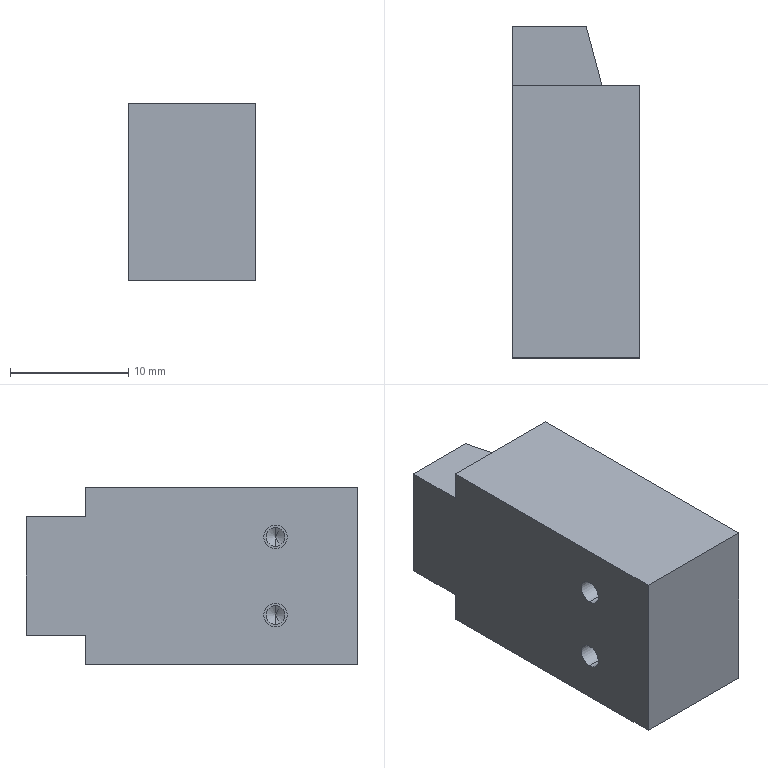Part | STEP file | 11-sy5120-5gz-01_sy51802operend-V2.0-V2.011_SingleA | 1 solid | 27 faces | box 10.8 x 28 x 15 mm | volume 4037 mm3 | plane 13 | cylinder 10 | cone 4 | commonest cylinder face diameters 1.6 x4 2 x4 3.4 x2
STEP:
#1=CARTESIAN_POINT('',(-5.119,6.95,-3.3));
#2=VERTEX_POINT('',#1);
#3=CARTESIAN_POINT('',(-5.6,6.95,-2.5));
#4=VERTEX_POINT('',#3);
#5=CARTESIAN_POINT('',(-5.6,6.95,-2.5));
#6=DIRECTION('',(-0.515,0.,0.8572));
#7=VECTOR('',#6,1000.);
#8=LINE('',#5,#7);
#9=EDGE_CURVE('',#2,#4,#8,.T.);
#10=ORIENTED_EDGE('',*,*,#9,.F.);
#11=CARTESIAN_POINT('',(-5.6,6.95,-4.1));
#12=VERTEX_POINT('',#11);
#13=CARTESIAN_POINT('',(-5.6,6.95,-4.1));
#14=DIRECTION('',(-0.515,0.,-0.8572));
#15=VECTOR('',#14,1000.);
#16=LINE('',#13,#15);
#17=EDGE_CURVE('',#2,#12,#16,.T.);
#18=ORIENTED_EDGE('',*,*,#17,.T.);
#19=CARTESIAN_POINT('',(-5.6,6.95,-3.3));
#20=DIRECTION('',(-1.,0.,0.));
#21=DIRECTION('',(0.,0.,1.));
#22=AXIS2_PLACEMENT_3D('',#19,#20,#21);
#23=CIRCLE('',#22,0.8);
#24=EDGE_CURVE('',#12,#4,#23,.T.);
#25=ORIENTED_EDGE('',*,*,#24,.T.);
#26=EDGE_LOOP('',(#10,#18,#25));
#27=FACE_OUTER_BOUND('',#26,.T.);
#28=CARTESIAN_POINT('',(-5.6,6.95,-3.3));
#29=DIRECTION('',(-1.,0.,0.));
#30=DIRECTION('',(0.,0.,1.));
#31=AXIS2_PLACEMENT_3D('',#28,#29,#30);
#32=CONICAL_SURFACE('',#31,0.8,1.03);
#33=ADVANCED_FACE('',(#27),#32,.F.);
#34=ORIENTED_EDGE('',*,*,#24,.F.);
#35=CARTESIAN_POINT('',(-6.8,6.95,-4.1));
#36=VERTEX_POINT('',#35);
#37=CARTESIAN_POINT('',(-10.8,6.95,-4.1));
#38=DIRECTION('',(-1.,0.,0.));
#39=VECTOR('',#38,1000.);
#40=LINE('',#37,#39);
#41=EDGE_CURVE('',#12,#36,#40,.T.);
#42=ORIENTED_EDGE('',*,*,#41,.T.);
#43=CARTESIAN_POINT('',(-6.8,6.95,-2.5));
#44=VERTEX_POINT('',#43);
#45=CARTESIAN_POINT('',(-6.8,6.95,-3.3));
#46=DIRECTION('',(-1.,0.,0.));
#47=DIRECTION('',(0.,0.,1.));
#48=AXIS2_PLACEMENT_3D('',#45,#46,#47);
#49=CIRCLE('',#48,0.8);
#50=EDGE_CURVE('',#36,#44,#49,.T.);
#51=ORIENTED_EDGE('',*,*,#50,.T.);
#52=CARTESIAN_POINT('',(-10.8,6.95,-2.5));
#53=DIRECTION('',(-1.,0.,0.));
#54=VECTOR('',#53,1000.);
#55=LINE('',#52,#54);
#56=EDGE_CURVE('',#4,#44,#55,.T.);
#57=ORIENTED_EDGE('',*,*,#56,.F.);
#58=EDGE_LOOP('',(#34,#42,#51,#57));
#59=FACE_OUTER_BOUND('',#58,.T.);
#60=CARTESIAN_POINT('',(-10.8,6.95,-3.3));
#61=DIRECTION('',(-1.,0.,0.));
#62=DIRECTION('',(0.,0.,1.));
#63=AXIS2_PLACEMENT_3D('',#60,#61,#62);
#64=CYLINDRICAL_SURFACE('',#63,0.8);
#65=ADVANCED_FACE('',(#59),#64,.F.);
#66=CARTESIAN_POINT('',(-6.8,6.95,-4.3));
#67=VERTEX_POINT('',#66);
#68=CARTESIAN_POINT('',(-6.8,6.95,-2.3));
#69=VERTEX_POINT('',#68);
#70=CARTESIAN_POINT('',(-6.8,6.95,-3.3));
#71=DIRECTION('',(-1.,0.,0.));
#72=DIRECTION('',(0.,0.,1.));
#73=AXIS2_PLACEMENT_3D('',#70,#71,#72);
#74=CIRCLE('',#73,1.);
#75=EDGE_CURVE('',#67,#69,#74,.T.);
#76=ORIENTED_EDGE('',*,*,#75,.F.);
#77=CARTESIAN_POINT('',(-10.8,6.95,-4.3));
#78=VERTEX_POINT('',#77);
#79=CARTESIAN_POINT('',(-10.8,6.95,-4.3));
#80=DIRECTION('',(-1.,0.,0.));
#81=VECTOR('',#80,1000.);
#82=LINE('',#79,#81);
#83=EDGE_CURVE('',#67,#78,#82,.T.);
#84=ORIENTED_EDGE('',*,*,#83,.T.);
#85=CARTESIAN_POINT('',(-10.8,6.95,-2.3));
#86=VERTEX_POINT('',#85);
#87=CARTESIAN_POINT('',(-10.8,6.95,-3.3));
#88=DIRECTION('',(-1.,0.,0.));
#89=DIRECTION('',(0.,0.,1.));
#90=AXIS2_PLACEMENT_3D('',#87,#88,#89);
#91=CIRCLE('',#90,1.);
#92=EDGE_CURVE('',#78,#86,#91,.T.);
#93=ORIENTED_EDGE('',*,*,#92,.T.);
#94=CARTESIAN_POINT('',(-10.8,6.95,-2.3));
#95=DIRECTION('',(-1.,0.,0.));
#96=VECTOR('',#95,1000.);
#97=LINE('',#94,#96);
#98=EDGE_CURVE('',#69,#86,#97,.T.);
#99=ORIENTED_EDGE('',*,*,#98,.F.);
#100=EDGE_LOOP('',(#76,#84,#93,#99));
#101=FACE_OUTER_BOUND('',#100,.T.);
#102=CARTESIAN_POINT('',(-10.8,6.95,-3.3));
#103=DIRECTION('',(-1.,0.,0.));
#104=DIRECTION('',(0.,0.,1.));
#105=AXIS2_PLACEMENT_3D('',#102,#103,#104);
#106=CYLINDRICAL_SURFACE('',#105,1.);
#107=ADVANCED_FACE('',(#101),#106,.F.);
#108=CARTESIAN_POINT('',(-5.119,6.95,3.3));
#109=VERTEX_POINT('',#108);
#110=CARTESIAN_POINT('',(-5.6,6.95,4.1));
#111=VERTEX_POINT('',#110);
#112=CARTESIAN_POINT('',(-5.6,6.95,4.1));
#113=DIRECTION('',(-0.515,0.,0.8572));
#114=VECTOR('',#113,1000.);
#115=LINE('',#112,#114);
#116=EDGE_CURVE('',#109,#111,#115,.T.);
#117=ORIENTED_EDGE('',*,*,#116,.F.);
#118=CARTESIAN_POINT('',(-5.6,6.95,2.5));
#119=VERTEX_POINT('',#118);
#120=CARTESIAN_POINT('',(-5.6,6.95,2.5));
#121=DIRECTION('',(-0.515,0.,-0.8572));
#122=VECTOR('',#121,1000.);
#123=LINE('',#120,#122);
#124=EDGE_CURVE('',#109,#119,#123,.T.);
#125=ORIENTED_EDGE('',*,*,#124,.T.);
#126=CARTESIAN_POINT('',(-5.6,6.95,3.3));
#127=DIRECTION('',(-1.,0.,0.));
#128=DIRECTION('',(0.,0.,1.));
#129=AXIS2_PLACEMENT_3D('',#126,#127,#128);
#130=CIRCLE('',#129,0.8);
#131=EDGE_CURVE('',#119,#111,#130,.T.);
#132=ORIENTED_EDGE('',*,*,#131,.T.);
#133=EDGE_LOOP('',(#117,#125,#132));
#134=FACE_OUTER_BOUND('',#133,.T.);
#135=CARTESIAN_POINT('',(-5.6,6.95,3.3));
#136=DIRECTION('',(-1.,0.,0.));
#137=DIRECTION('',(0.,0.,1.));
#138=AXIS2_PLACEMENT_3D('',#135,#136,#137);
#139=CONICAL_SURFACE('',#138,0.8,1.03);
#140=ADVANCED_FACE('',(#134),#139,.F.);
#141=ORIENTED_EDGE('',*,*,#131,.F.);
#142=CARTESIAN_POINT('',(-6.8,6.95,2.5));
#143=VERTEX_POINT('',#142);
#144=CARTESIAN_POINT('',(-10.8,6.95,2.5));
#145=DIRECTION('',(-1.,0.,0.));
#146=VECTOR('',#145,1000.);
#147=LINE('',#144,#146);
#148=EDGE_CURVE('',#119,#143,#147,.T.);
#149=ORIENTED_EDGE('',*,*,#148,.T.);
#150=CARTESIAN_POINT('',(-6.8,6.95,4.1));
#151=VERTEX_POINT('',#150);
#152=CARTESIAN_POINT('',(-6.8,6.95,3.3));
#153=DIRECTION('',(-1.,0.,0.));
#154=DIRECTION('',(0.,0.,1.));
#155=AXIS2_PLACEMENT_3D('',#152,#153,#154);
#156=CIRCLE('',#155,0.8);
#157=EDGE_CURVE('',#143,#151,#156,.T.);
#158=ORIENTED_EDGE('',*,*,#157,.T.);
#159=CARTESIAN_POINT('',(-10.8,6.95,4.1));
#160=DIRECTION('',(-1.,0.,0.));
#161=VECTOR('',#160,1000.);
#162=LINE('',#159,#161);
#163=EDGE_CURVE('',#111,#151,#162,.T.);
#164=ORIENTED_EDGE('',*,*,#163,.F.);
#165=EDGE_LOOP('',(#141,#149,#158,#164));
#166=FACE_OUTER_BOUND('',#165,.T.);
#167=CARTESIAN_POINT('',(-10.8,6.95,3.3));
#168=DIRECTION('',(-1.,0.,0.));
#169=DIRECTION('',(0.,0.,1.));
#170=AXIS2_PLACEMENT_3D('',#167,#168,#169);
#171=CYLINDRICAL_SURFACE('',#170,0.8);
#172=ADVANCED_FACE('',(#166),#171,.F.);
#173=CARTESIAN_POINT('',(-6.8,6.95,2.3));
#174=VERTEX_POINT('',#173);
#175=CARTESIAN_POINT('',(-6.8,6.95,4.3));
#176=VERTEX_POINT('',#175);
#177=CARTESIAN_POINT('',(-6.8,6.95,3.3));
#178=DIRECTION('',(-1.,0.,0.));
#179=DIRECTION('',(0.,0.,1.));
#180=AXIS2_PLACEMENT_3D('',#177,#178,#179);
#181=CIRCLE('',#180,1.);
#182=EDGE_CURVE('',#174,#176,#181,.T.);
#183=ORIENTED_EDGE('',*,*,#182,.F.);
#184=CARTESIAN_POINT('',(-10.8,6.95,2.3));
#185=VERTEX_POINT('',#184);
#186=CARTESIAN_POINT('',(-10.8,6.95,2.3));
#187=DIRECTION('',(-1.,0.,0.));
#188=VECTOR('',#187,1000.);
#189=LINE('',#186,#188);
#190=EDGE_CURVE('',#174,#185,#189,.T.);
#191=ORIENTED_EDGE('',*,*,#190,.T.);
#192=CARTESIAN_POINT('',(-10.8,6.95,4.3));
#193=VERTEX_POINT('',#192);
#194=CARTESIAN_POINT('',(-10.8,6.95,3.3));
#195=DIRECTION('',(-1.,0.,0.));
#196=DIRECTION('',(0.,0.,1.));
#197=AXIS2_PLACEMENT_3D('',#194,#195,#196);
#198=CIRCLE('',#197,1.);
#199=EDGE_CURVE('',#185,#193,#198,.T.);
#200=ORIENTED_EDGE('',*,*,#199,.T.);
#201=CARTESIAN_POINT('',(-10.8,6.95,4.3));
#202=DIRECTION('',(-1.,0.,0.));
#203=VECTOR('',#202,1000.);
#204=LINE('',#201,#203);
#205=EDGE_CURVE('',#176,#193,#204,.T.);
#206=ORIENTED_EDGE('',*,*,#205,.F.);
#207=EDGE_LOOP('',(#183,#191,#200,#206));
#208=FACE_OUTER_BOUND('',#207,.T.);
#209=CARTESIAN_POINT('',(-10.8,6.95,3.3));
#210=DIRECTION('',(-1.,0.,0.));
#211=DIRECTION('',(0.,0.,1.));
#212=AXIS2_PLACEMENT_3D('',#209,#210,#211);
#213=CYLINDRICAL_SURFACE('',#212,1.);
#214=ADVANCED_FACE('',(#208),#213,.F.);
#215=CARTESIAN_POINT('',(-8.1,27.5,-1.7));
#216=VERTEX_POINT('',#215);
#217=CARTESIAN_POINT('',(-8.1,27.5,1.7));
#218=VERTEX_POINT('',#217);
#219=CARTESIAN_POINT('',(-8.1,27.5,0.));
#220=DIRECTION('',(0.,1.,0.));
#221=DIRECTION('',(0.,0.,1.));
#222=AXIS2_PLACEMENT_3D('',#219,#220,#221);
#223=CIRCLE('',#222,1.7);
#224=EDGE_CURVE('',#216,#218,#223,.T.);
#225=ORIENTED_EDGE('',*,*,#224,.F.);
#226=CARTESIAN_POINT('',(-8.1,28.,-1.7));
#227=VERTEX_POINT('',#226);
#228=CARTESIAN_POINT('',(-8.1,27.5,-1.7));
#229=DIRECTION('',(0.,1.,0.));
#230=VECTOR('',#229,1000.);
#231=LINE('',#228,#230);
#232=EDGE_CURVE('',#216,#227,#231,.T.);
#233=ORIENTED_EDGE('',*,*,#232,.T.);
#234=CARTESIAN_POINT('',(-8.1,28.,1.7));
#235=VERTEX_POINT('',#234);
#236=CARTESIAN_POINT('',(-8.1,28.,0.));
#237=DIRECTION('',(0.,1.,0.));
#238=DIRECTION('',(0.,0.,1.));
#239=AXIS2_PLACEMENT_3D('',#236,#237,#238);
#240=CIRCLE('',#239,1.7);
#241=EDGE_CURVE('',#227,#235,#240,.T.);
#242=ORIENTED_EDGE('',*,*,#241,.T.);
#243=CARTESIAN_POINT('',(-8.1,27.5,1.7));
#244=DIRECTION('',(0.,1.,0.));
#245=VECTOR('',#244,1000.);
#246=LINE('',#243,#245);
#247=EDGE_CURVE('',#218,#235,#246,.T.);
#248=ORIENTED_EDGE('',*,*,#247,.F.);
#249=EDGE_LOOP('',(#225,#233,#242,#248));
#250=FACE_OUTER_BOUND('',#249,.T.);
#251=CARTESIAN_POINT('',(-8.1,27.5,0.));
#252=DIRECTION('',(0.,1.,0.));
#253=DIRECTION('',(0.,0.,1.));
#254=AXIS2_PLACEMENT_3D('',#251,#252,#253);
#255=CYLINDRICAL_SURFACE('',#254,1.7);
#256=ADVANCED_FACE('',(#250),#255,.F.);
#257=CARTESIAN_POINT('',(-10.8,0.,7.5));
#258=VERTEX_POINT('',#257);
#259=CARTESIAN_POINT('',(-10.8,0.,-7.5));
#260=VERTEX_POINT('',#259);
#261=CARTESIAN_POINT('',(-10.8,0.,7.5));
#262=DIRECTION('',(0.,0.,-1.));
#263=VECTOR('',#262,1000.);
#264=LINE('',#261,#263);
#265=EDGE_CURVE('',#258,#260,#264,.T.);
#266=ORIENTED_EDGE('',*,*,#265,.T.);
#267=CARTESIAN_POINT('',(0.,0.,-7.5));
#268=VERTEX_POINT('',#267);
#269=CARTESIAN_POINT('',(-10.8,0.,-7.5));
#270=DIRECTION('',(1.,0.,0.));
#271=VECTOR('',#270,1000.);
#272=LINE('',#269,#271);
#273=EDGE_CURVE('',#260,#268,#272,.T.);
#274=ORIENTED_EDGE('',*,*,#273,.T.);
#275=CARTESIAN_POINT('',(0.,0.,7.5));
#276=VERTEX_POINT('',#275);
#277=CARTESIAN_POINT('',(0.,0.,7.5));
#278=DIRECTION('',(0.,0.,-1.));
#279=VECTOR('',#278,1000.);
#280=LINE('',#277,#279);
#281=EDGE_CURVE('',#276,#268,#280,.T.);
#282=ORIENTED_EDGE('',*,*,#281,.F.);
#283=CARTESIAN_POINT('',(-10.8,0.,7.5));
#284=DIRECTION('',(1.,0.,0.));
#285=VECTOR('',#284,1000.);
#286=LINE('',#283,#285);
#287=EDGE_CURVE('',#258,#276,#286,.T.);
#288=ORIENTED_EDGE('',*,*,#287,.F.);
#289=EDGE_LOOP('',(#266,#274,#282,#288));
#290=FACE_OUTER_BOUND('',#289,.T.);
#291=CARTESIAN_POINT('',(-10.8,0.,7.5));
#292=DIRECTION('',(0.,1.,0.));
#293=DIRECTION('',(0.,0.,1.));
#294=AXIS2_PLACEMENT_3D('',#291,#292,#293);
#295=PLANE('',#294);
#296=ADVANCED_FACE('',(#290),#295,.F.);
#297=ORIENTED_EDGE('',*,*,#281,.T.);
#298=CARTESIAN_POINT('',(0.,23.,-7.5));
#299=VERTEX_POINT('',#298);
#300=CARTESIAN_POINT('',(0.,0.,-7.5));
#301=DIRECTION('',(0.,1.,0.));
#302=VECTOR('',#301,1000.);
#303=LINE('',#300,#302);
#304=EDGE_CURVE('',#268,#299,#303,.T.);
#305=ORIENTED_EDGE('',*,*,#304,.T.);
#306=CARTESIAN_POINT('',(0.,23.,7.5));
#307=VERTEX_POINT('',#306);
#308=CARTESIAN_POINT('',(0.,23.,7.5));
#309=DIRECTION('',(0.,0.,-1.));
#310=VECTOR('',#309,1000.);
#311=LINE('',#308,#310);
#312=EDGE_CURVE('',#307,#299,#311,.T.);
#313=ORIENTED_EDGE('',*,*,#312,.F.);
#314=CARTESIAN_POINT('',(0.,0.,7.5));
#315=DIRECTION('',(0.,1.,0.));
#316=VECTOR('',#315,1000.);
#317=LINE('',#314,#316);
#318=EDGE_CURVE('',#276,#307,#317,.T.);
#319=ORIENTED_EDGE('',*,*,#318,.F.);
#320=EDGE_LOOP('',(#297,#305,#313,#319));
#321=FACE_OUTER_BOUND('',#320,.T.);
#322=CARTESIAN_POINT('',(0.,0.,7.5));
#323=DIRECTION('',(-1.,0.,0.));
#324=DIRECTION('',(0.,-1.,0.));
#325=AXIS2_PLACEMENT_3D('',#322,#323,#324);
#326=PLANE('',#325);
#327=ADVANCED_FACE('',(#321),#326,.F.);
#328=CARTESIAN_POINT('',(-10.8,23.,-5.));
#329=VERTEX_POINT('',#328);
#330=CARTESIAN_POINT('',(-10.8,23.,-7.5));
#331=VERTEX_POINT('',#330);
#332=CARTESIAN_POINT('',(-10.8,23.,7.5));
#333=DIRECTION('',(0.,0.,-1.));
#334=VECTOR('',#333,1000.);
#335=LINE('',#332,#334);
#336=EDGE_CURVE('',#329,#331,#335,.T.);
#337=ORIENTED_EDGE('',*,*,#336,.F.);
#338=CARTESIAN_POINT('',(-3.2,23.,-5.));
#339=VERTEX_POINT('',#338);
#340=CARTESIAN_POINT('',(-3.2,23.,-5.));
#341=DIRECTION('',(1.,0.,0.));
#342=VECTOR('',#341,1000.);
#343=LINE('',#340,#342);
#344=EDGE_CURVE('',#329,#339,#343,.T.);
#345=ORIENTED_EDGE('',*,*,#344,.T.);
#346=CARTESIAN_POINT('',(-3.2,23.,5.));
#347=VERTEX_POINT('',#346);
#348=CARTESIAN_POINT('',(-3.2,23.,5.));
#349=DIRECTION('',(0.,0.,-1.));
#350=VECTOR('',#349,1000.);
#351=LINE('',#348,#350);
#352=EDGE_CURVE('',#347,#339,#351,.T.);
#353=ORIENTED_EDGE('',*,*,#352,.F.);
#354=CARTESIAN_POINT('',(-10.8,23.,5.));
#355=VERTEX_POINT('',#354);
#356=CARTESIAN_POINT('',(-3.2,23.,5.));
#357=DIRECTION('',(1.,0.,0.));
#358=VECTOR('',#357,1000.);
#359=LINE('',#356,#358);
#360=EDGE_CURVE('',#355,#347,#359,.T.);
#361=ORIENTED_EDGE('',*,*,#360,.F.);
#362=CARTESIAN_POINT('',(-10.8,23.,7.5));
#363=VERTEX_POINT('',#362);
#364=CARTESIAN_POINT('',(-10.8,23.,7.5));
#365=DIRECTION('',(0.,0.,-1.));
#366=VECTOR('',#365,1000.);
#367=LINE('',#364,#366);
#368=EDGE_CURVE('',#363,#355,#367,.T.);
#369=ORIENTED_EDGE('',*,*,#368,.F.);
#370=CARTESIAN_POINT('',(0.,23.,7.5));
#371=DIRECTION('',(-1.,0.,0.));
#372=VECTOR('',#371,1000.);
#373=LINE('',#370,#372);
#374=EDGE_CURVE('',#307,#363,#373,.T.);
#375=ORIENTED_EDGE('',*,*,#374,.F.);
#376=ORIENTED_EDGE('',*,*,#312,.T.);
#377=CARTESIAN_POINT('',(0.,23.,-7.5));
#378=DIRECTION('',(-1.,0.,0.));
#379=VECTOR('',#378,1000.);
#380=LINE('',#377,#379);
#381=EDGE_CURVE('',#299,#331,#380,.T.);
#382=ORIENTED_EDGE('',*,*,#381,.T.);
#383=EDGE_LOOP('',(#337,#345,#353,#361,#369,#375,#376,#382));
#384=FACE_OUTER_BOUND('',#383,.T.);
#385=CARTESIAN_POINT('',(0.,23.,7.5));
#386=DIRECTION('',(0.,-1.,0.));
#387=DIRECTION('',(1.,0.,0.));
#388=AXIS2_PLACEMENT_3D('',#385,#386,#387);
#389=PLANE('',#388);
#390=ADVANCED_FACE('',(#384),#389,.F.);
#391=CARTESIAN_POINT('',(-10.8,6.95,-3.3));
#392=DIRECTION('',(-1.,0.,0.));
#393=DIRECTION('',(0.,0.,1.));
#394=AXIS2_PLACEMENT_3D('',#391,#392,#393);
#395=CIRCLE('',#394,1.);
#396=EDGE_CURVE('',#86,#78,#395,.T.);
#397=ORIENTED_EDGE('',*,*,#396,.F.);
#398=ORIENTED_EDGE('',*,*,#92,.F.);
#399=EDGE_LOOP('',(#397,#398));
#400=FACE_BOUND('',#399,.T.);
#401=CARTESIAN_POINT('',(-10.8,6.95,3.3));
#402=DIRECTION('',(-1.,0.,0.));
#403=DIRECTION('',(0.,0.,1.));
#404=AXIS2_PLACEMENT_3D('',#401,#402,#403);
#405=CIRCLE('',#404,1.);
#406=EDGE_CURVE('',#193,#185,#405,.T.);
#407=ORIENTED_EDGE('',*,*,#406,.F.);
#408=ORIENTED_EDGE('',*,*,#199,.F.);
#409=EDGE_LOOP('',(#407,#408));
#410=FACE_BOUND('',#409,.T.);
#411=ORIENTED_EDGE('',*,*,#368,.T.);
#412=CARTESIAN_POINT('',(-10.8,28.,5.));
#413=VERTEX_POINT('',#412);
#414=CARTESIAN_POINT('',(-10.8,23.,5.));
#415=DIRECTION('',(0.,-1.,0.));
#416=VECTOR('',#415,1000.);
#417=LINE('',#414,#416);
#418=EDGE_CURVE('',#413,#355,#417,.T.);
#419=ORIENTED_EDGE('',*,*,#418,.F.);
#420=CARTESIAN_POINT('',(-10.8,28.,-5.));
#421=VERTEX_POINT('',#420);
#422=CARTESIAN_POINT('',(-10.8,28.,5.));
#423=DIRECTION('',(0.,0.,-1.));
#424=VECTOR('',#423,1000.);
#425=LINE('',#422,#424);
#426=EDGE_CURVE('',#413,#421,#425,.T.);
#427=ORIENTED_EDGE('',*,*,#426,.T.);
#428=CARTESIAN_POINT('',(-10.8,23.,-5.));
#429=DIRECTION('',(0.,-1.,0.));
#430=VECTOR('',#429,1000.);
#431=LINE('',#428,#430);
#432=EDGE_CURVE('',#421,#329,#431,.T.);
#433=ORIENTED_EDGE('',*,*,#432,.T.);
#434=ORIENTED_EDGE('',*,*,#336,.T.);
#435=CARTESIAN_POINT('',(-10.8,23.,-7.5));
#436=DIRECTION('',(0.,-1.,0.));
#437=VECTOR('',#436,1000.);
#438=LINE('',#435,#437);
#439=EDGE_CURVE('',#331,#260,#438,.T.);
#440=ORIENTED_EDGE('',*,*,#439,.T.);
#441=ORIENTED_EDGE('',*,*,#265,.F.);
#442=CARTESIAN_POINT('',(-10.8,23.,7.5));
#443=DIRECTION('',(0.,-1.,0.));
#444=VECTOR('',#443,1000.);
#445=LINE('',#442,#444);
#446=EDGE_CURVE('',#363,#258,#445,.T.);
#447=ORIENTED_EDGE('',*,*,#446,.F.);
#448=EDGE_LOOP('',(#411,#419,#427,#433,#434,#440,#441,#447));
#449=FACE_OUTER_BOUND('',#448,.T.);
#450=CARTESIAN_POINT('',(-10.8,23.,7.5));
#451=DIRECTION('',(1.,0.,0.));
#452=DIRECTION('',(0.,1.,0.));
#453=AXIS2_PLACEMENT_3D('',#450,#451,#452);
#454=PLANE('',#453);
#455=ADVANCED_FACE('',(#400,#410,#449),#454,.F.);
#456=ORIENTED_EDGE('',*,*,#287,.T.);
#457=ORIENTED_EDGE('',*,*,#318,.T.);
#458=ORIENTED_EDGE('',*,*,#374,.T.);
#459=ORIENTED_EDGE('',*,*,#446,.T.);
#460=EDGE_LOOP('',(#456,#457,#458,#459));
#461=FACE_OUTER_BOUND('',#460,.T.);
#462=CARTESIAN_POINT('',(-10.8,0.,7.5));
#463=DIRECTION('',(0.,0.,-1.));
#464=DIRECTION('',(-1.,0.,0.));
#465=AXIS2_PLACEMENT_3D('',#462,#463,#464);
#466=PLANE('',#465);
#467=ADVANCED_FACE('',(#461),#466,.F.);
#468=ORIENTED_EDGE('',*,*,#273,.F.);
#469=ORIENTED_EDGE('',*,*,#439,.F.);
#470=ORIENTED_EDGE('',*,*,#381,.F.);
#471=ORIENTED_EDGE('',*,*,#304,.F.);
#472=EDGE_LOOP('',(#468,#469,#470,#471));
#473=FACE_OUTER_BOUND('',#472,.T.);
#474=CARTESIAN_POINT('',(-10.8,0.,-7.5));
#475=DIRECTION('',(0.,0.,-1.));
#476=DIRECTION('',(-1.,0.,0.));
#477=AXIS2_PLACEMENT_3D('',#474,#475,#476);
#478=PLANE('',#477);
#479=ADVANCED_FACE('',(#473),#478,.T.);
#480=CARTESIAN_POINT('',(-4.54,28.,-5.));
#481=VERTEX_POINT('',#480);
#482=CARTESIAN_POINT('',(-4.54,28.,-5.));
#483=DIRECTION('',(-0.2588,0.9659,0.));
#484=VECTOR('',#483,1000.);
#485=LINE('',#482,#484);
#486=EDGE_CURVE('',#339,#481,#485,.T.);
#487=ORIENTED_EDGE('',*,*,#486,.T.);
#488=CARTESIAN_POINT('',(-4.54,28.,5.));
#489=VERTEX_POINT('',#488);
#490=CARTESIAN_POINT('',(-4.54,28.,5.));
#491=DIRECTION('',(0.,0.,-1.));
#492=VECTOR('',#491,1000.);
#493=LINE('',#490,#492);
#494=EDGE_CURVE('',#489,#481,#493,.T.);
#495=ORIENTED_EDGE('',*,*,#494,.F.);
#496=CARTESIAN_POINT('',(-4.54,28.,5.));
#497=DIRECTION('',(-0.2588,0.9659,0.));
#498=VECTOR('',#497,1000.);
#499=LINE('',#496,#498);
#500=EDGE_CURVE('',#347,#489,#499,.T.);
#501=ORIENTED_EDGE('',*,*,#500,.F.);
#502=ORIENTED_EDGE('',*,*,#352,.T.);
#503=EDGE_LOOP('',(#487,#495,#501,#502));
#504=FACE_OUTER_BOUND('',#503,.T.);
#505=CARTESIAN_POINT('',(-4.54,28.,5.));
#506=DIRECTION('',(-0.9659,-0.2588,0.));
#507=DIRECTION('',(0.2588,-0.9659,0.));
#508=AXIS2_PLACEMENT_3D('',#505,#506,#507);
#509=PLANE('',#508);
#510=ADVANCED_FACE('',(#504),#509,.F.);
#511=CARTESIAN_POINT('',(-8.1,28.,0.));
#512=DIRECTION('',(0.,1.,0.));
#513=DIRECTION('',(0.,0.,1.));
#514=AXIS2_PLACEMENT_3D('',#511,#512,#513);
#515=CIRCLE('',#514,1.7);
#516=EDGE_CURVE('',#235,#227,#515,.T.);
#517=ORIENTED_EDGE('',*,*,#516,.F.);
#518=ORIENTED_EDGE('',*,*,#241,.F.);
#519=EDGE_LOOP('',(#517,#518));
#520=FACE_BOUND('',#519,.T.);
#521=CARTESIAN_POINT('',(-10.8,28.,-5.));
#522=DIRECTION('',(-1.,0.,0.));
#523=VECTOR('',#522,1000.);
#524=LINE('',#521,#523);
#525=EDGE_CURVE('',#481,#421,#524,.T.);
#526=ORIENTED_EDGE('',*,*,#525,.T.);
#527=ORIENTED_EDGE('',*,*,#426,.F.);
#528=CARTESIAN_POINT('',(-10.8,28.,5.));
#529=DIRECTION('',(-1.,0.,0.));
#530=VECTOR('',#529,1000.);
#531=LINE('',#528,#530);
#532=EDGE_CURVE('',#489,#413,#531,.T.);
#533=ORIENTED_EDGE('',*,*,#532,.F.);
#534=ORIENTED_EDGE('',*,*,#494,.T.);
#535=EDGE_LOOP('',(#526,#527,#533,#534));
#536=FACE_OUTER_BOUND('',#535,.T.);
#537=CARTESIAN_POINT('',(-10.8,28.,5.));
#538=DIRECTION('',(0.,-1.,0.));
#539=DIRECTION('',(1.,0.,0.));
#540=AXIS2_PLACEMENT_3D('',#537,#538,#539);
#541=PLANE('',#540);
#542=ADVANCED_FACE('',(#520,#536),#541,.F.);
#543=ORIENTED_EDGE('',*,*,#418,.T.);
#544=ORIENTED_EDGE('',*,*,#360,.T.);
#545=ORIENTED_EDGE('',*,*,#500,.T.);
#546=ORIENTED_EDGE('',*,*,#532,.T.);
#547=EDGE_LOOP('',(#543,#544,#545,#546));
#548=FACE_OUTER_BOUND('',#547,.T.);
#549=CARTESIAN_POINT('',(-10.8,28.,5.));
#550=DIRECTION('',(0.,0.,-1.));
#551=DIRECTION('',(-1.,0.,0.));
#552=AXIS2_PLACEMENT_3D('',#549,#550,#551);
#553=PLANE('',#552);
#554=ADVANCED_FACE('',(#548),#553,.F.);
#555=ORIENTED_EDGE('',*,*,#432,.F.);
#556=ORIENTED_EDGE('',*,*,#525,.F.);
#557=ORIENTED_EDGE('',*,*,#486,.F.);
#558=ORIENTED_EDGE('',*,*,#344,.F.);
#559=EDGE_LOOP('',(#555,#556,#557,#558));
#560=FACE_OUTER_BOUND('',#559,.T.);
#561=CARTESIAN_POINT('',(-10.8,28.,-5.));
#562=DIRECTION('',(0.,0.,-1.));
#563=DIRECTION('',(-1.,0.,0.));
#564=AXIS2_PLACEMENT_3D('',#561,#562,#563);
#565=PLANE('',#564);
#566=ADVANCED_FACE('',(#560),#565,.T.);
#567=ORIENTED_EDGE('',*,*,#232,.F.);
#568=CARTESIAN_POINT('',(-8.1,27.5,0.));
#569=DIRECTION('',(0.,1.,0.));
#570=DIRECTION('',(0.,0.,1.));
#571=AXIS2_PLACEMENT_3D('',#568,#569,#570);
#572=CIRCLE('',#571,1.7);
#573=EDGE_CURVE('',#218,#216,#572,.T.);
#574=ORIENTED_EDGE('',*,*,#573,.F.);
#575=ORIENTED_EDGE('',*,*,#247,.T.);
#576=ORIENTED_EDGE('',*,*,#516,.T.);
#577=EDGE_LOOP('',(#567,#574,#575,#576));
#578=FACE_OUTER_BOUND('',#577,.T.);
#579=CARTESIAN_POINT('',(-8.1,27.5,0.));
#580=DIRECTION('',(0.,1.,0.));
#581=DIRECTION('',(0.,0.,1.));
#582=AXIS2_PLACEMENT_3D('',#579,#580,#581);
#583=CYLINDRICAL_SURFACE('',#582,1.7);
#584=ADVANCED_FACE('',(#578),#583,.F.);
#585=ORIENTED_EDGE('',*,*,#573,.T.);
#586=ORIENTED_EDGE('',*,*,#224,.T.);
#587=EDGE_LOOP('',(#585,#586));
#588=FACE_OUTER_BOUND('',#587,.T.);
#589=CARTESIAN_POINT('',(-8.1,27.5,0.));
#590=DIRECTION('',(0.,1.,0.));
#591=DIRECTION('',(0.,0.,1.));
#592=AXIS2_PLACEMENT_3D('',#589,#590,#591);
#593=PLANE('',#592);
#594=ADVANCED_FACE('',(#588),#593,.T.);
#595=ORIENTED_EDGE('',*,*,#190,.F.);
#596=CARTESIAN_POINT('',(-6.8,6.95,3.3));
#597=DIRECTION('',(-1.,0.,0.));
#598=DIRECTION('',(0.,0.,1.));
#599=AXIS2_PLACEMENT_3D('',#596,#597,#598);
#600=CIRCLE('',#599,1.);
#601=EDGE_CURVE('',#176,#174,#600,.T.);
#602=ORIENTED_EDGE('',*,*,#601,.F.);
#603=ORIENTED_EDGE('',*,*,#205,.T.);
#604=ORIENTED_EDGE('',*,*,#406,.T.);
#605=EDGE_LOOP('',(#595,#602,#603,#604));
#606=FACE_OUTER_BOUND('',#605,.T.);
#607=CARTESIAN_POINT('',(-10.8,6.95,3.3));
#608=DIRECTION('',(-1.,0.,0.));
#609=DIRECTION('',(0.,0.,1.));
#610=AXIS2_PLACEMENT_3D('',#607,#608,#609);
#611=CYLINDRICAL_SURFACE('',#610,1.);
#612=ADVANCED_FACE('',(#606),#611,.F.);
#613=CARTESIAN_POINT('',(-6.8,6.95,3.3));
#614=DIRECTION('',(-1.,0.,0.));
#615=DIRECTION('',(0.,0.,1.));
#616=AXIS2_PLACEMENT_3D('',#613,#614,#615);
#617=CIRCLE('',#616,0.8);
#618=EDGE_CURVE('',#151,#143,#617,.T.);
#619=ORIENTED_EDGE('',*,*,#618,.F.);
#620=ORIENTED_EDGE('',*,*,#157,.F.);
#621=EDGE_LOOP('',(#619,#620));
#622=FACE_BOUND('',#621,.T.);
#623=ORIENTED_EDGE('',*,*,#601,.T.);
#624=ORIENTED_EDGE('',*,*,#182,.T.);
#625=EDGE_LOOP('',(#623,#624));
#626=FACE_OUTER_BOUND('',#625,.T.);
#627=CARTESIAN_POINT('',(-6.8,7.75,3.3));
#628=DIRECTION('',(1.,0.,0.));
#629=DIRECTION('',(0.,0.,-1.));
#630=AXIS2_PLACEMENT_3D('',#627,#628,#629);
#631=PLANE('',#630);
#632=ADVANCED_FACE('',(#622,#626),#631,.F.);
#633=ORIENTED_EDGE('',*,*,#148,.F.);
#634=CARTESIAN_POINT('',(-5.6,6.95,3.3));
#635=DIRECTION('',(-1.,0.,0.));
#636=DIRECTION('',(0.,0.,1.));
#637=AXIS2_PLACEMENT_3D('',#634,#635,#636);
#638=CIRCLE('',#637,0.8);
#639=EDGE_CURVE('',#111,#119,#638,.T.);
#640=ORIENTED_EDGE('',*,*,#639,.F.);
#641=ORIENTED_EDGE('',*,*,#163,.T.);
#642=ORIENTED_EDGE('',*,*,#618,.T.);
#643=EDGE_LOOP('',(#633,#640,#641,#642));
#644=FACE_OUTER_BOUND('',#643,.T.);
#645=CARTESIAN_POINT('',(-10.8,6.95,3.3));
#646=DIRECTION('',(-1.,0.,0.));
#647=DIRECTION('',(0.,0.,1.));
#648=AXIS2_PLACEMENT_3D('',#645,#646,#647);
#649=CYLINDRICAL_SURFACE('',#648,0.8);
#650=ADVANCED_FACE('',(#644),#649,.F.);
#651=ORIENTED_EDGE('',*,*,#124,.F.);
#652=ORIENTED_EDGE('',*,*,#116,.T.);
#653=ORIENTED_EDGE('',*,*,#639,.T.);
#654=EDGE_LOOP('',(#651,#652,#653));
#655=FACE_OUTER_BOUND('',#654,.T.);
#656=CARTESIAN_POINT('',(-5.6,6.95,3.3));
#657=DIRECTION('',(-1.,0.,0.));
#658=DIRECTION('',(0.,0.,1.));
#659=AXIS2_PLACEMENT_3D('',#656,#657,#658);
#660=CONICAL_SURFACE('',#659,0.8,1.03);
#661=ADVANCED_FACE('',(#655),#660,.F.);
#662=ORIENTED_EDGE('',*,*,#83,.F.);
#663=CARTESIAN_POINT('',(-6.8,6.95,-3.3));
#664=DIRECTION('',(-1.,0.,0.));
#665=DIRECTION('',(0.,0.,1.));
#666=AXIS2_PLACEMENT_3D('',#663,#664,#665);
#667=CIRCLE('',#666,1.);
#668=EDGE_CURVE('',#69,#67,#667,.T.);
#669=ORIENTED_EDGE('',*,*,#668,.F.);
#670=ORIENTED_EDGE('',*,*,#98,.T.);
#671=ORIENTED_EDGE('',*,*,#396,.T.);
#672=EDGE_LOOP('',(#662,#669,#670,#671));
#673=FACE_OUTER_BOUND('',#672,.T.);
#674=CARTESIAN_POINT('',(-10.8,6.95,-3.3));
#675=DIRECTION('',(-1.,0.,0.));
#676=DIRECTION('',(0.,0.,1.));
#677=AXIS2_PLACEMENT_3D('',#674,#675,#676);
#678=CYLINDRICAL_SURFACE('',#677,1.);
#679=ADVANCED_FACE('',(#673),#678,.F.);
#680=CARTESIAN_POINT('',(-6.8,6.95,-3.3));
#681=DIRECTION('',(-1.,0.,0.));
#682=DIRECTION('',(0.,0.,1.));
#683=AXIS2_PLACEMENT_3D('',#680,#681,#682);
#684=CIRCLE('',#683,0.8);
#685=EDGE_CURVE('',#44,#36,#684,.T.);
#686=ORIENTED_EDGE('',*,*,#685,.F.);
#687=ORIENTED_EDGE('',*,*,#50,.F.);
#688=EDGE_LOOP('',(#686,#687));
#689=FACE_BOUND('',#688,.T.);
#690=ORIENTED_EDGE('',*,*,#668,.T.);
#691=ORIENTED_EDGE('',*,*,#75,.T.);
#692=EDGE_LOOP('',(#690,#691));
#693=FACE_OUTER_BOUND('',#692,.T.);
#694=CARTESIAN_POINT('',(-6.8,7.75,-3.3));
#695=DIRECTION('',(1.,0.,0.));
#696=DIRECTION('',(0.,0.,-1.));
#697=AXIS2_PLACEMENT_3D('',#694,#695,#696);
#698=PLANE('',#697);
#699=ADVANCED_FACE('',(#689,#693),#698,.F.);
#700=ORIENTED_EDGE('',*,*,#41,.F.);
#701=CARTESIAN_POINT('',(-5.6,6.95,-3.3));
#702=DIRECTION('',(-1.,0.,0.));
#703=DIRECTION('',(0.,0.,1.));
#704=AXIS2_PLACEMENT_3D('',#701,#702,#703);
#705=CIRCLE('',#704,0.8);
#706=EDGE_CURVE('',#4,#12,#705,.T.);
#707=ORIENTED_EDGE('',*,*,#706,.F.);
#708=ORIENTED_EDGE('',*,*,#56,.T.);
#709=ORIENTED_EDGE('',*,*,#685,.T.);
#710=EDGE_LOOP('',(#700,#707,#708,#709));
#711=FACE_OUTER_BOUND('',#710,.T.);
#712=CARTESIAN_POINT('',(-10.8,6.95,-3.3));
#713=DIRECTION('',(-1.,0.,0.));
#714=DIRECTION('',(0.,0.,1.));
#715=AXIS2_PLACEMENT_3D('',#712,#713,#714);
#716=CYLINDRICAL_SURFACE('',#715,0.8);
#717=ADVANCED_FACE('',(#711),#716,.F.);
#718=ORIENTED_EDGE('',*,*,#17,.F.);
#719=ORIENTED_EDGE('',*,*,#9,.T.);
#720=ORIENTED_EDGE('',*,*,#706,.T.);
#721=EDGE_LOOP('',(#718,#719,#720));
#722=FACE_OUTER_BOUND('',#721,.T.);
#723=CARTESIAN_POINT('',(-5.6,6.95,-3.3));
#724=DIRECTION('',(-1.,0.,0.));
#725=DIRECTION('',(0.,0.,1.));
#726=AXIS2_PLACEMENT_3D('',#723,#724,#725);
#727=CONICAL_SURFACE('',#726,0.8,1.03);
#728=ADVANCED_FACE('',(#722),#727,.F.);
#729=CLOSED_SHELL('',(#33,#65,#107,#140,#172,#214,#256,#296,#327,#390,#455,#467,#479,#510,#542,#554,#566,#584,#594,#612,#632,#650,#661,#679,#699,#717,#728));
#730=MANIFOLD_SOLID_BREP('',#729);
#731=CARTESIAN_POINT('',(0.,0.,0.));
#732=DIRECTION('',(0.,0.,1.));
#733=DIRECTION('',(1.,0.,0.));
#734=AXIS2_PLACEMENT_3D('',#731,#732,#733);
#735=(LENGTH_UNIT()NAMED_UNIT(*)SI_UNIT(.MILLI.,.METRE.));
#736=UNCERTAINTY_MEASURE_WITH_UNIT(LENGTH_MEASURE(0.00001),#735,'','');
#737=(NAMED_UNIT(*)PLANE_ANGLE_UNIT()SI_UNIT($,.RADIAN.));
#738=(NAMED_UNIT(*)SI_UNIT($,.STERADIAN.)SOLID_ANGLE_UNIT());
#739=(GEOMETRIC_REPRESENTATION_CONTEXT(3)GLOBAL_UNCERTAINTY_ASSIGNED_CONTEXT((#736))GLOBAL_UNIT_ASSIGNED_CONTEXT((#735,#737,#738))REPRESENTATION_CONTEXT('',''));
#740=ADVANCED_BREP_SHAPE_REPRESENTATION('',(#730,#734),#739);